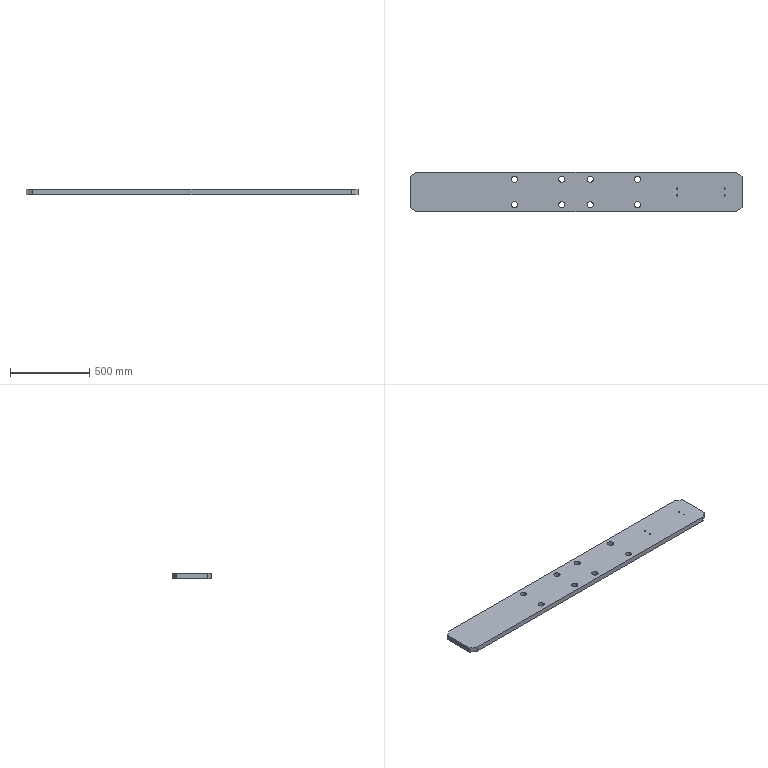Part | SolidWorks | features Extrusion 1, HoleWzd 1, LPattern 1 | 1 solid | 34 faces | box 2100 x 250 x 32 mm | volume 16420254 mm3 | cylinder 24 | plane 10 | commonest cylinder face diameters 39 x16 6.8 x8
STEP:
#1=CARTESIAN_POINT('',(936.6,-22.,-16.));
#2=VERTEX_POINT('',#1);
#3=CARTESIAN_POINT('',(943.4,-22.,-16.));
#4=VERTEX_POINT('',#3);
#5=CARTESIAN_POINT('',(940.,-22.,-16.));
#6=DIRECTION('',(0.,0.,1.));
#7=DIRECTION('',(1.,0.,0.));
#8=AXIS2_PLACEMENT_3D('',#5,#6,#7);
#9=CIRCLE('',#8,3.4);
#10=EDGE_CURVE('',#2,#4,#9,.T.);
#11=ORIENTED_EDGE('',*,*,#10,.F.);
#12=CARTESIAN_POINT('',(936.6,-22.,16.));
#13=VERTEX_POINT('',#12);
#14=CARTESIAN_POINT('',(936.6,-22.,16.));
#15=DIRECTION('',(0.,0.,1.));
#16=VECTOR('',#15,1000.);
#17=LINE('',#14,#16);
#18=EDGE_CURVE('',#2,#13,#17,.T.);
#19=ORIENTED_EDGE('',*,*,#18,.T.);
#20=CARTESIAN_POINT('',(943.4,-22.,16.));
#21=VERTEX_POINT('',#20);
#22=CARTESIAN_POINT('',(940.,-22.,16.));
#23=DIRECTION('',(0.,0.,1.));
#24=DIRECTION('',(1.,0.,0.));
#25=AXIS2_PLACEMENT_3D('',#22,#23,#24);
#26=CIRCLE('',#25,3.4);
#27=EDGE_CURVE('',#13,#21,#26,.T.);
#28=ORIENTED_EDGE('',*,*,#27,.T.);
#29=CARTESIAN_POINT('',(943.4,-22.,16.));
#30=DIRECTION('',(0.,0.,1.));
#31=VECTOR('',#30,1000.);
#32=LINE('',#29,#31);
#33=EDGE_CURVE('',#4,#21,#32,.T.);
#34=ORIENTED_EDGE('',*,*,#33,.F.);
#35=EDGE_LOOP('',(#11,#19,#28,#34));
#36=FACE_OUTER_BOUND('',#35,.T.);
#37=CARTESIAN_POINT('',(940.,-22.,16.));
#38=DIRECTION('',(0.,0.,1.));
#39=DIRECTION('',(1.,0.,0.));
#40=AXIS2_PLACEMENT_3D('',#37,#38,#39);
#41=CYLINDRICAL_SURFACE('',#40,3.4);
#42=ADVANCED_FACE('',(#36),#41,.F.);
#43=CARTESIAN_POINT('',(636.6,-22.,-16.));
#44=VERTEX_POINT('',#43);
#45=CARTESIAN_POINT('',(643.4,-22.,-16.));
#46=VERTEX_POINT('',#45);
#47=CARTESIAN_POINT('',(640.,-22.,-16.));
#48=DIRECTION('',(0.,0.,1.));
#49=DIRECTION('',(1.,0.,0.));
#50=AXIS2_PLACEMENT_3D('',#47,#48,#49);
#51=CIRCLE('',#50,3.4);
#52=EDGE_CURVE('',#44,#46,#51,.T.);
#53=ORIENTED_EDGE('',*,*,#52,.F.);
#54=CARTESIAN_POINT('',(636.6,-22.,16.));
#55=VERTEX_POINT('',#54);
#56=CARTESIAN_POINT('',(636.6,-22.,16.));
#57=DIRECTION('',(0.,0.,1.));
#58=VECTOR('',#57,1000.);
#59=LINE('',#56,#58);
#60=EDGE_CURVE('',#44,#55,#59,.T.);
#61=ORIENTED_EDGE('',*,*,#60,.T.);
#62=CARTESIAN_POINT('',(643.4,-22.,16.));
#63=VERTEX_POINT('',#62);
#64=CARTESIAN_POINT('',(640.,-22.,16.));
#65=DIRECTION('',(0.,0.,1.));
#66=DIRECTION('',(1.,0.,0.));
#67=AXIS2_PLACEMENT_3D('',#64,#65,#66);
#68=CIRCLE('',#67,3.4);
#69=EDGE_CURVE('',#55,#63,#68,.T.);
#70=ORIENTED_EDGE('',*,*,#69,.T.);
#71=CARTESIAN_POINT('',(643.4,-22.,16.));
#72=DIRECTION('',(0.,0.,1.));
#73=VECTOR('',#72,1000.);
#74=LINE('',#71,#73);
#75=EDGE_CURVE('',#46,#63,#74,.T.);
#76=ORIENTED_EDGE('',*,*,#75,.F.);
#77=EDGE_LOOP('',(#53,#61,#70,#76));
#78=FACE_OUTER_BOUND('',#77,.T.);
#79=CARTESIAN_POINT('',(640.,-22.,16.));
#80=DIRECTION('',(0.,0.,1.));
#81=DIRECTION('',(1.,0.,0.));
#82=AXIS2_PLACEMENT_3D('',#79,#80,#81);
#83=CYLINDRICAL_SURFACE('',#82,3.4);
#84=ADVANCED_FACE('',(#78),#83,.F.);
#85=CARTESIAN_POINT('',(936.6,22.,-16.));
#86=VERTEX_POINT('',#85);
#87=CARTESIAN_POINT('',(943.4,22.,-16.));
#88=VERTEX_POINT('',#87);
#89=CARTESIAN_POINT('',(940.,22.,-16.));
#90=DIRECTION('',(0.,0.,1.));
#91=DIRECTION('',(1.,0.,0.));
#92=AXIS2_PLACEMENT_3D('',#89,#90,#91);
#93=CIRCLE('',#92,3.4);
#94=EDGE_CURVE('',#86,#88,#93,.T.);
#95=ORIENTED_EDGE('',*,*,#94,.F.);
#96=CARTESIAN_POINT('',(936.6,22.,16.));
#97=VERTEX_POINT('',#96);
#98=CARTESIAN_POINT('',(936.6,22.,16.));
#99=DIRECTION('',(0.,0.,1.));
#100=VECTOR('',#99,1000.);
#101=LINE('',#98,#100);
#102=EDGE_CURVE('',#86,#97,#101,.T.);
#103=ORIENTED_EDGE('',*,*,#102,.T.);
#104=CARTESIAN_POINT('',(943.4,22.,16.));
#105=VERTEX_POINT('',#104);
#106=CARTESIAN_POINT('',(940.,22.,16.));
#107=DIRECTION('',(0.,0.,1.));
#108=DIRECTION('',(1.,0.,0.));
#109=AXIS2_PLACEMENT_3D('',#106,#107,#108);
#110=CIRCLE('',#109,3.4);
#111=EDGE_CURVE('',#97,#105,#110,.T.);
#112=ORIENTED_EDGE('',*,*,#111,.T.);
#113=CARTESIAN_POINT('',(943.4,22.,16.));
#114=DIRECTION('',(0.,0.,1.));
#115=VECTOR('',#114,1000.);
#116=LINE('',#113,#115);
#117=EDGE_CURVE('',#88,#105,#116,.T.);
#118=ORIENTED_EDGE('',*,*,#117,.F.);
#119=EDGE_LOOP('',(#95,#103,#112,#118));
#120=FACE_OUTER_BOUND('',#119,.T.);
#121=CARTESIAN_POINT('',(940.,22.,16.));
#122=DIRECTION('',(0.,0.,1.));
#123=DIRECTION('',(1.,0.,0.));
#124=AXIS2_PLACEMENT_3D('',#121,#122,#123);
#125=CYLINDRICAL_SURFACE('',#124,3.4);
#126=ADVANCED_FACE('',(#120),#125,.F.);
#127=CARTESIAN_POINT('',(636.6,22.,-16.));
#128=VERTEX_POINT('',#127);
#129=CARTESIAN_POINT('',(643.4,22.,-16.));
#130=VERTEX_POINT('',#129);
#131=CARTESIAN_POINT('',(640.,22.,-16.));
#132=DIRECTION('',(0.,0.,1.));
#133=DIRECTION('',(1.,0.,0.));
#134=AXIS2_PLACEMENT_3D('',#131,#132,#133);
#135=CIRCLE('',#134,3.4);
#136=EDGE_CURVE('',#128,#130,#135,.T.);
#137=ORIENTED_EDGE('',*,*,#136,.F.);
#138=CARTESIAN_POINT('',(636.6,22.,16.));
#139=VERTEX_POINT('',#138);
#140=CARTESIAN_POINT('',(636.6,22.,16.));
#141=DIRECTION('',(0.,0.,1.));
#142=VECTOR('',#141,1000.);
#143=LINE('',#140,#142);
#144=EDGE_CURVE('',#128,#139,#143,.T.);
#145=ORIENTED_EDGE('',*,*,#144,.T.);
#146=CARTESIAN_POINT('',(643.4,22.,16.));
#147=VERTEX_POINT('',#146);
#148=CARTESIAN_POINT('',(640.,22.,16.));
#149=DIRECTION('',(0.,0.,1.));
#150=DIRECTION('',(1.,0.,0.));
#151=AXIS2_PLACEMENT_3D('',#148,#149,#150);
#152=CIRCLE('',#151,3.4);
#153=EDGE_CURVE('',#139,#147,#152,.T.);
#154=ORIENTED_EDGE('',*,*,#153,.T.);
#155=CARTESIAN_POINT('',(643.4,22.,16.));
#156=DIRECTION('',(0.,0.,1.));
#157=VECTOR('',#156,1000.);
#158=LINE('',#155,#157);
#159=EDGE_CURVE('',#130,#147,#158,.T.);
#160=ORIENTED_EDGE('',*,*,#159,.F.);
#161=EDGE_LOOP('',(#137,#145,#154,#160));
#162=FACE_OUTER_BOUND('',#161,.T.);
#163=CARTESIAN_POINT('',(640.,22.,16.));
#164=DIRECTION('',(0.,0.,1.));
#165=DIRECTION('',(1.,0.,0.));
#166=AXIS2_PLACEMENT_3D('',#163,#164,#165);
#167=CYLINDRICAL_SURFACE('',#166,3.4);
#168=ADVANCED_FACE('',(#162),#167,.F.);
#169=CARTESIAN_POINT('',(370.5,80.,16.));
#170=VERTEX_POINT('',#169);
#171=CARTESIAN_POINT('',(409.5,80.,16.));
#172=VERTEX_POINT('',#171);
#173=CARTESIAN_POINT('',(390.,80.,16.));
#174=DIRECTION('',(0.,0.,1.));
#175=DIRECTION('',(-1.,0.,0.));
#176=AXIS2_PLACEMENT_3D('',#173,#174,#175);
#177=CIRCLE('',#176,19.5);
#178=EDGE_CURVE('',#170,#172,#177,.T.);
#179=ORIENTED_EDGE('',*,*,#178,.T.);
#180=CARTESIAN_POINT('',(409.5,80.,-16.));
#181=VERTEX_POINT('',#180);
#182=CARTESIAN_POINT('',(409.5,80.,16.));
#183=DIRECTION('',(0.,0.,-1.));
#184=VECTOR('',#183,1000.);
#185=LINE('',#182,#184);
#186=EDGE_CURVE('',#172,#181,#185,.T.);
#187=ORIENTED_EDGE('',*,*,#186,.T.);
#188=CARTESIAN_POINT('',(370.5,80.,-16.));
#189=VERTEX_POINT('',#188);
#190=CARTESIAN_POINT('',(390.,80.,-16.));
#191=DIRECTION('',(0.,0.,1.));
#192=DIRECTION('',(-1.,0.,0.));
#193=AXIS2_PLACEMENT_3D('',#190,#191,#192);
#194=CIRCLE('',#193,19.5);
#195=EDGE_CURVE('',#189,#181,#194,.T.);
#196=ORIENTED_EDGE('',*,*,#195,.F.);
#197=CARTESIAN_POINT('',(370.5,80.,16.));
#198=DIRECTION('',(0.,0.,-1.));
#199=VECTOR('',#198,1000.);
#200=LINE('',#197,#199);
#201=EDGE_CURVE('',#170,#189,#200,.T.);
#202=ORIENTED_EDGE('',*,*,#201,.F.);
#203=EDGE_LOOP('',(#179,#187,#196,#202));
#204=FACE_OUTER_BOUND('',#203,.T.);
#205=CARTESIAN_POINT('',(390.,80.,16.));
#206=DIRECTION('',(0.,0.,-1.));
#207=DIRECTION('',(-1.,0.,0.));
#208=AXIS2_PLACEMENT_3D('',#205,#206,#207);
#209=CYLINDRICAL_SURFACE('',#208,19.5);
#210=ADVANCED_FACE('',(#204),#209,.F.);
#211=CARTESIAN_POINT('',(70.5,80.,16.));
#212=VERTEX_POINT('',#211);
#213=CARTESIAN_POINT('',(109.5,80.,16.));
#214=VERTEX_POINT('',#213);
#215=CARTESIAN_POINT('',(90.,80.,16.));
#216=DIRECTION('',(0.,0.,1.));
#217=DIRECTION('',(-1.,0.,0.));
#218=AXIS2_PLACEMENT_3D('',#215,#216,#217);
#219=CIRCLE('',#218,19.5);
#220=EDGE_CURVE('',#212,#214,#219,.T.);
#221=ORIENTED_EDGE('',*,*,#220,.T.);
#222=CARTESIAN_POINT('',(109.5,80.,-16.));
#223=VERTEX_POINT('',#222);
#224=CARTESIAN_POINT('',(109.5,80.,16.));
#225=DIRECTION('',(0.,0.,-1.));
#226=VECTOR('',#225,1000.);
#227=LINE('',#224,#226);
#228=EDGE_CURVE('',#214,#223,#227,.T.);
#229=ORIENTED_EDGE('',*,*,#228,.T.);
#230=CARTESIAN_POINT('',(70.5,80.,-16.));
#231=VERTEX_POINT('',#230);
#232=CARTESIAN_POINT('',(90.,80.,-16.));
#233=DIRECTION('',(0.,0.,1.));
#234=DIRECTION('',(-1.,0.,0.));
#235=AXIS2_PLACEMENT_3D('',#232,#233,#234);
#236=CIRCLE('',#235,19.5);
#237=EDGE_CURVE('',#231,#223,#236,.T.);
#238=ORIENTED_EDGE('',*,*,#237,.F.);
#239=CARTESIAN_POINT('',(70.5,80.,16.));
#240=DIRECTION('',(0.,0.,-1.));
#241=VECTOR('',#240,1000.);
#242=LINE('',#239,#241);
#243=EDGE_CURVE('',#212,#231,#242,.T.);
#244=ORIENTED_EDGE('',*,*,#243,.F.);
#245=EDGE_LOOP('',(#221,#229,#238,#244));
#246=FACE_OUTER_BOUND('',#245,.T.);
#247=CARTESIAN_POINT('',(90.,80.,16.));
#248=DIRECTION('',(0.,0.,-1.));
#249=DIRECTION('',(-1.,0.,0.));
#250=AXIS2_PLACEMENT_3D('',#247,#248,#249);
#251=CYLINDRICAL_SURFACE('',#250,19.5);
#252=ADVANCED_FACE('',(#246),#251,.F.);
#253=CARTESIAN_POINT('',(70.5,-80.,16.));
#254=VERTEX_POINT('',#253);
#255=CARTESIAN_POINT('',(109.5,-80.,16.));
#256=VERTEX_POINT('',#255);
#257=CARTESIAN_POINT('',(90.,-80.,16.));
#258=DIRECTION('',(0.,0.,1.));
#259=DIRECTION('',(1.,0.,0.));
#260=AXIS2_PLACEMENT_3D('',#257,#258,#259);
#261=CIRCLE('',#260,19.5);
#262=EDGE_CURVE('',#254,#256,#261,.T.);
#263=ORIENTED_EDGE('',*,*,#262,.T.);
#264=CARTESIAN_POINT('',(109.5,-80.,-16.));
#265=VERTEX_POINT('',#264);
#266=CARTESIAN_POINT('',(109.5,-80.,16.));
#267=DIRECTION('',(0.,0.,-1.));
#268=VECTOR('',#267,1000.);
#269=LINE('',#266,#268);
#270=EDGE_CURVE('',#256,#265,#269,.T.);
#271=ORIENTED_EDGE('',*,*,#270,.T.);
#272=CARTESIAN_POINT('',(70.5,-80.,-16.));
#273=VERTEX_POINT('',#272);
#274=CARTESIAN_POINT('',(90.,-80.,-16.));
#275=DIRECTION('',(0.,0.,1.));
#276=DIRECTION('',(1.,0.,0.));
#277=AXIS2_PLACEMENT_3D('',#274,#275,#276);
#278=CIRCLE('',#277,19.5);
#279=EDGE_CURVE('',#273,#265,#278,.T.);
#280=ORIENTED_EDGE('',*,*,#279,.F.);
#281=CARTESIAN_POINT('',(70.5,-80.,16.));
#282=DIRECTION('',(0.,0.,-1.));
#283=VECTOR('',#282,1000.);
#284=LINE('',#281,#283);
#285=EDGE_CURVE('',#254,#273,#284,.T.);
#286=ORIENTED_EDGE('',*,*,#285,.F.);
#287=EDGE_LOOP('',(#263,#271,#280,#286));
#288=FACE_OUTER_BOUND('',#287,.T.);
#289=CARTESIAN_POINT('',(90.,-80.,16.));
#290=DIRECTION('',(0.,0.,-1.));
#291=DIRECTION('',(-1.,0.,0.));
#292=AXIS2_PLACEMENT_3D('',#289,#290,#291);
#293=CYLINDRICAL_SURFACE('',#292,19.5);
#294=ADVANCED_FACE('',(#288),#293,.F.);
#295=CARTESIAN_POINT('',(370.5,-80.,16.));
#296=VERTEX_POINT('',#295);
#297=CARTESIAN_POINT('',(409.5,-80.,16.));
#298=VERTEX_POINT('',#297);
#299=CARTESIAN_POINT('',(390.,-80.,16.));
#300=DIRECTION('',(0.,0.,1.));
#301=DIRECTION('',(1.,0.,0.));
#302=AXIS2_PLACEMENT_3D('',#299,#300,#301);
#303=CIRCLE('',#302,19.5);
#304=EDGE_CURVE('',#296,#298,#303,.T.);
#305=ORIENTED_EDGE('',*,*,#304,.T.);
#306=CARTESIAN_POINT('',(409.5,-80.,-16.));
#307=VERTEX_POINT('',#306);
#308=CARTESIAN_POINT('',(409.5,-80.,16.));
#309=DIRECTION('',(0.,0.,-1.));
#310=VECTOR('',#309,1000.);
#311=LINE('',#308,#310);
#312=EDGE_CURVE('',#298,#307,#311,.T.);
#313=ORIENTED_EDGE('',*,*,#312,.T.);
#314=CARTESIAN_POINT('',(370.5,-80.,-16.));
#315=VERTEX_POINT('',#314);
#316=CARTESIAN_POINT('',(390.,-80.,-16.));
#317=DIRECTION('',(0.,0.,1.));
#318=DIRECTION('',(1.,0.,0.));
#319=AXIS2_PLACEMENT_3D('',#316,#317,#318);
#320=CIRCLE('',#319,19.5);
#321=EDGE_CURVE('',#315,#307,#320,.T.);
#322=ORIENTED_EDGE('',*,*,#321,.F.);
#323=CARTESIAN_POINT('',(370.5,-80.,16.));
#324=DIRECTION('',(0.,0.,-1.));
#325=VECTOR('',#324,1000.);
#326=LINE('',#323,#325);
#327=EDGE_CURVE('',#296,#315,#326,.T.);
#328=ORIENTED_EDGE('',*,*,#327,.F.);
#329=EDGE_LOOP('',(#305,#313,#322,#328));
#330=FACE_OUTER_BOUND('',#329,.T.);
#331=CARTESIAN_POINT('',(390.,-80.,16.));
#332=DIRECTION('',(0.,0.,-1.));
#333=DIRECTION('',(-1.,0.,0.));
#334=AXIS2_PLACEMENT_3D('',#331,#332,#333);
#335=CYLINDRICAL_SURFACE('',#334,19.5);
#336=ADVANCED_FACE('',(#330),#335,.F.);
#337=CARTESIAN_POINT('',(-409.5,-80.,16.));
#338=VERTEX_POINT('',#337);
#339=CARTESIAN_POINT('',(-370.5,-80.,16.));
#340=VERTEX_POINT('',#339);
#341=CARTESIAN_POINT('',(-390.,-80.,16.));
#342=DIRECTION('',(0.,0.,1.));
#343=DIRECTION('',(-1.,0.,0.));
#344=AXIS2_PLACEMENT_3D('',#341,#342,#343);
#345=CIRCLE('',#344,19.5);
#346=EDGE_CURVE('',#338,#340,#345,.T.);
#347=ORIENTED_EDGE('',*,*,#346,.T.);
#348=CARTESIAN_POINT('',(-370.5,-80.,-16.));
#349=VERTEX_POINT('',#348);
#350=CARTESIAN_POINT('',(-370.5,-80.,16.));
#351=DIRECTION('',(0.,0.,-1.));
#352=VECTOR('',#351,1000.);
#353=LINE('',#350,#352);
#354=EDGE_CURVE('',#340,#349,#353,.T.);
#355=ORIENTED_EDGE('',*,*,#354,.T.);
#356=CARTESIAN_POINT('',(-409.5,-80.,-16.));
#357=VERTEX_POINT('',#356);
#358=CARTESIAN_POINT('',(-390.,-80.,-16.));
#359=DIRECTION('',(0.,0.,1.));
#360=DIRECTION('',(-1.,0.,0.));
#361=AXIS2_PLACEMENT_3D('',#358,#359,#360);
#362=CIRCLE('',#361,19.5);
#363=EDGE_CURVE('',#357,#349,#362,.T.);
#364=ORIENTED_EDGE('',*,*,#363,.F.);
#365=CARTESIAN_POINT('',(-409.5,-80.,16.));
#366=DIRECTION('',(0.,0.,-1.));
#367=VECTOR('',#366,1000.);
#368=LINE('',#365,#367);
#369=EDGE_CURVE('',#338,#357,#368,.T.);
#370=ORIENTED_EDGE('',*,*,#369,.F.);
#371=EDGE_LOOP('',(#347,#355,#364,#370));
#372=FACE_OUTER_BOUND('',#371,.T.);
#373=CARTESIAN_POINT('',(-390.,-80.,16.));
#374=DIRECTION('',(0.,0.,-1.));
#375=DIRECTION('',(-1.,0.,0.));
#376=AXIS2_PLACEMENT_3D('',#373,#374,#375);
#377=CYLINDRICAL_SURFACE('',#376,19.5);
#378=ADVANCED_FACE('',(#372),#377,.F.);
#379=CARTESIAN_POINT('',(-109.5,-80.,16.));
#380=VERTEX_POINT('',#379);
#381=CARTESIAN_POINT('',(-70.5,-80.,16.));
#382=VERTEX_POINT('',#381);
#383=CARTESIAN_POINT('',(-90.,-80.,16.));
#384=DIRECTION('',(0.,0.,1.));
#385=DIRECTION('',(-1.,0.,0.));
#386=AXIS2_PLACEMENT_3D('',#383,#384,#385);
#387=CIRCLE('',#386,19.5);
#388=EDGE_CURVE('',#380,#382,#387,.T.);
#389=ORIENTED_EDGE('',*,*,#388,.T.);
#390=CARTESIAN_POINT('',(-70.5,-80.,-16.));
#391=VERTEX_POINT('',#390);
#392=CARTESIAN_POINT('',(-70.5,-80.,16.));
#393=DIRECTION('',(0.,0.,-1.));
#394=VECTOR('',#393,1000.);
#395=LINE('',#392,#394);
#396=EDGE_CURVE('',#382,#391,#395,.T.);
#397=ORIENTED_EDGE('',*,*,#396,.T.);
#398=CARTESIAN_POINT('',(-109.5,-80.,-16.));
#399=VERTEX_POINT('',#398);
#400=CARTESIAN_POINT('',(-90.,-80.,-16.));
#401=DIRECTION('',(0.,0.,1.));
#402=DIRECTION('',(-1.,0.,0.));
#403=AXIS2_PLACEMENT_3D('',#400,#401,#402);
#404=CIRCLE('',#403,19.5);
#405=EDGE_CURVE('',#399,#391,#404,.T.);
#406=ORIENTED_EDGE('',*,*,#405,.F.);
#407=CARTESIAN_POINT('',(-109.5,-80.,16.));
#408=DIRECTION('',(0.,0.,-1.));
#409=VECTOR('',#408,1000.);
#410=LINE('',#407,#409);
#411=EDGE_CURVE('',#380,#399,#410,.T.);
#412=ORIENTED_EDGE('',*,*,#411,.F.);
#413=EDGE_LOOP('',(#389,#397,#406,#412));
#414=FACE_OUTER_BOUND('',#413,.T.);
#415=CARTESIAN_POINT('',(-90.,-80.,16.));
#416=DIRECTION('',(0.,0.,-1.));
#417=DIRECTION('',(-1.,0.,0.));
#418=AXIS2_PLACEMENT_3D('',#415,#416,#417);
#419=CYLINDRICAL_SURFACE('',#418,19.5);
#420=ADVANCED_FACE('',(#414),#419,.F.);
#421=CARTESIAN_POINT('',(-109.5,80.,16.));
#422=VERTEX_POINT('',#421);
#423=CARTESIAN_POINT('',(-70.5,80.,16.));
#424=VERTEX_POINT('',#423);
#425=CARTESIAN_POINT('',(-90.,80.,16.));
#426=DIRECTION('',(0.,0.,1.));
#427=DIRECTION('',(1.,0.,0.));
#428=AXIS2_PLACEMENT_3D('',#425,#426,#427);
#429=CIRCLE('',#428,19.5);
#430=EDGE_CURVE('',#422,#424,#429,.T.);
#431=ORIENTED_EDGE('',*,*,#430,.T.);
#432=CARTESIAN_POINT('',(-70.5,80.,-16.));
#433=VERTEX_POINT('',#432);
#434=CARTESIAN_POINT('',(-70.5,80.,16.));
#435=DIRECTION('',(0.,0.,-1.));
#436=VECTOR('',#435,1000.);
#437=LINE('',#434,#436);
#438=EDGE_CURVE('',#424,#433,#437,.T.);
#439=ORIENTED_EDGE('',*,*,#438,.T.);
#440=CARTESIAN_POINT('',(-109.5,80.,-16.));
#441=VERTEX_POINT('',#440);
#442=CARTESIAN_POINT('',(-90.,80.,-16.));
#443=DIRECTION('',(0.,0.,1.));
#444=DIRECTION('',(1.,0.,0.));
#445=AXIS2_PLACEMENT_3D('',#442,#443,#444);
#446=CIRCLE('',#445,19.5);
#447=EDGE_CURVE('',#441,#433,#446,.T.);
#448=ORIENTED_EDGE('',*,*,#447,.F.);
#449=CARTESIAN_POINT('',(-109.5,80.,16.));
#450=DIRECTION('',(0.,0.,-1.));
#451=VECTOR('',#450,1000.);
#452=LINE('',#449,#451);
#453=EDGE_CURVE('',#422,#441,#452,.T.);
#454=ORIENTED_EDGE('',*,*,#453,.F.);
#455=EDGE_LOOP('',(#431,#439,#448,#454));
#456=FACE_OUTER_BOUND('',#455,.T.);
#457=CARTESIAN_POINT('',(-90.,80.,16.));
#458=DIRECTION('',(0.,0.,-1.));
#459=DIRECTION('',(-1.,0.,0.));
#460=AXIS2_PLACEMENT_3D('',#457,#458,#459);
#461=CYLINDRICAL_SURFACE('',#460,19.5);
#462=ADVANCED_FACE('',(#456),#461,.F.);
#463=CARTESIAN_POINT('',(-409.5,80.,16.));
#464=VERTEX_POINT('',#463);
#465=CARTESIAN_POINT('',(-370.5,80.,16.));
#466=VERTEX_POINT('',#465);
#467=CARTESIAN_POINT('',(-390.,80.,16.));
#468=DIRECTION('',(0.,0.,1.));
#469=DIRECTION('',(1.,0.,0.));
#470=AXIS2_PLACEMENT_3D('',#467,#468,#469);
#471=CIRCLE('',#470,19.5);
#472=EDGE_CURVE('',#464,#466,#471,.T.);
#473=ORIENTED_EDGE('',*,*,#472,.T.);
#474=CARTESIAN_POINT('',(-370.5,80.,-16.));
#475=VERTEX_POINT('',#474);
#476=CARTESIAN_POINT('',(-370.5,80.,16.));
#477=DIRECTION('',(0.,0.,-1.));
#478=VECTOR('',#477,1000.);
#479=LINE('',#476,#478);
#480=EDGE_CURVE('',#466,#475,#479,.T.);
#481=ORIENTED_EDGE('',*,*,#480,.T.);
#482=CARTESIAN_POINT('',(-409.5,80.,-16.));
#483=VERTEX_POINT('',#482);
#484=CARTESIAN_POINT('',(-390.,80.,-16.));
#485=DIRECTION('',(0.,0.,1.));
#486=DIRECTION('',(1.,0.,0.));
#487=AXIS2_PLACEMENT_3D('',#484,#485,#486);
#488=CIRCLE('',#487,19.5);
#489=EDGE_CURVE('',#483,#475,#488,.T.);
#490=ORIENTED_EDGE('',*,*,#489,.F.);
#491=CARTESIAN_POINT('',(-409.5,80.,16.));
#492=DIRECTION('',(0.,0.,-1.));
#493=VECTOR('',#492,1000.);
#494=LINE('',#491,#493);
#495=EDGE_CURVE('',#464,#483,#494,.T.);
#496=ORIENTED_EDGE('',*,*,#495,.F.);
#497=EDGE_LOOP('',(#473,#481,#490,#496));
#498=FACE_OUTER_BOUND('',#497,.T.);
#499=CARTESIAN_POINT('',(-390.,80.,16.));
#500=DIRECTION('',(0.,0.,-1.));
#501=DIRECTION('',(-1.,0.,0.));
#502=AXIS2_PLACEMENT_3D('',#499,#500,#501);
#503=CYLINDRICAL_SURFACE('',#502,19.5);
#504=ADVANCED_FACE('',(#498),#503,.F.);
#505=CARTESIAN_POINT('',(940.,22.,16.));
#506=DIRECTION('',(0.,0.,1.));
#507=DIRECTION('',(1.,0.,0.));
#508=AXIS2_PLACEMENT_3D('',#505,#506,#507);
#509=CIRCLE('',#508,3.4);
#510=EDGE_CURVE('',#105,#97,#509,.T.);
#511=ORIENTED_EDGE('',*,*,#510,.F.);
#512=ORIENTED_EDGE('',*,*,#111,.F.);
#513=EDGE_LOOP('',(#511,#512));
#514=FACE_BOUND('',#513,.T.);
#515=CARTESIAN_POINT('',(640.,22.,16.));
#516=DIRECTION('',(0.,0.,1.));
#517=DIRECTION('',(1.,0.,0.));
#518=AXIS2_PLACEMENT_3D('',#515,#516,#517);
#519=CIRCLE('',#518,3.4);
#520=EDGE_CURVE('',#147,#139,#519,.T.);
#521=ORIENTED_EDGE('',*,*,#520,.F.);
#522=ORIENTED_EDGE('',*,*,#153,.F.);
#523=EDGE_LOOP('',(#521,#522));
#524=FACE_BOUND('',#523,.T.);
#525=ORIENTED_EDGE('',*,*,#220,.F.);
#526=CARTESIAN_POINT('',(90.,80.,16.));
#527=DIRECTION('',(0.,0.,1.));
#528=DIRECTION('',(-1.,0.,0.));
#529=AXIS2_PLACEMENT_3D('',#526,#527,#528);
#530=CIRCLE('',#529,19.5);
#531=EDGE_CURVE('',#214,#212,#530,.T.);
#532=ORIENTED_EDGE('',*,*,#531,.F.);
#533=EDGE_LOOP('',(#525,#532));
#534=FACE_BOUND('',#533,.T.);
#535=ORIENTED_EDGE('',*,*,#304,.F.);
#536=CARTESIAN_POINT('',(390.,-80.,16.));
#537=DIRECTION('',(0.,0.,1.));
#538=DIRECTION('',(1.,0.,0.));
#539=AXIS2_PLACEMENT_3D('',#536,#537,#538);
#540=CIRCLE('',#539,19.5);
#541=EDGE_CURVE('',#298,#296,#540,.T.);
#542=ORIENTED_EDGE('',*,*,#541,.F.);
#543=EDGE_LOOP('',(#535,#542));
#544=FACE_BOUND('',#543,.T.);
#545=ORIENTED_EDGE('',*,*,#388,.F.);
#546=CARTESIAN_POINT('',(-90.,-80.,16.));
#547=DIRECTION('',(0.,0.,1.));
#548=DIRECTION('',(-1.,0.,0.));
#549=AXIS2_PLACEMENT_3D('',#546,#547,#548);
#550=CIRCLE('',#549,19.5);
#551=EDGE_CURVE('',#382,#380,#550,.T.);
#552=ORIENTED_EDGE('',*,*,#551,.F.);
#553=EDGE_LOOP('',(#545,#552));
#554=FACE_BOUND('',#553,.T.);
#555=ORIENTED_EDGE('',*,*,#472,.F.);
#556=CARTESIAN_POINT('',(-390.,80.,16.));
#557=DIRECTION('',(0.,0.,1.));
#558=DIRECTION('',(1.,0.,0.));
#559=AXIS2_PLACEMENT_3D('',#556,#557,#558);
#560=CIRCLE('',#559,19.5);
#561=EDGE_CURVE('',#466,#464,#560,.T.);
#562=ORIENTED_EDGE('',*,*,#561,.F.);
#563=EDGE_LOOP('',(#555,#562));
#564=FACE_BOUND('',#563,.T.);
#565=CARTESIAN_POINT('',(1006.699,-125.,16.));
#566=VERTEX_POINT('',#565);
#567=CARTESIAN_POINT('',(1050.,-100.,16.));
#568=VERTEX_POINT('',#567);
#569=CARTESIAN_POINT('',(1050.,-100.,16.));
#570=DIRECTION('',(0.866,0.5,0.));
#571=VECTOR('',#570,1000.);
#572=LINE('',#569,#571);
#573=EDGE_CURVE('',#566,#568,#572,.T.);
#574=ORIENTED_EDGE('',*,*,#573,.T.);
#575=CARTESIAN_POINT('',(1050.,100.,16.));
#576=VERTEX_POINT('',#575);
#577=CARTESIAN_POINT('',(1050.,100.,16.));
#578=DIRECTION('',(0.,1.,0.));
#579=VECTOR('',#578,1000.);
#580=LINE('',#577,#579);
#581=EDGE_CURVE('',#568,#576,#580,.T.);
#582=ORIENTED_EDGE('',*,*,#581,.T.);
#583=CARTESIAN_POINT('',(1006.699,125.,16.));
#584=VERTEX_POINT('',#583);
#585=CARTESIAN_POINT('',(1050.,100.,16.));
#586=DIRECTION('',(-0.866,0.5,0.));
#587=VECTOR('',#586,1000.);
#588=LINE('',#585,#587);
#589=EDGE_CURVE('',#576,#584,#588,.T.);
#590=ORIENTED_EDGE('',*,*,#589,.T.);
#591=CARTESIAN_POINT('',(-1006.699,125.,16.));
#592=VERTEX_POINT('',#591);
#593=CARTESIAN_POINT('',(-1006.699,125.,16.));
#594=DIRECTION('',(-1.,0.,0.));
#595=VECTOR('',#594,1000.);
#596=LINE('',#593,#595);
#597=EDGE_CURVE('',#584,#592,#596,.T.);
#598=ORIENTED_EDGE('',*,*,#597,.T.);
#599=CARTESIAN_POINT('',(-1050.,100.,16.));
#600=VERTEX_POINT('',#599);
#601=CARTESIAN_POINT('',(-1050.,100.,16.));
#602=DIRECTION('',(-0.866,-0.5,0.));
#603=VECTOR('',#602,1000.);
#604=LINE('',#601,#603);
#605=EDGE_CURVE('',#592,#600,#604,.T.);
#606=ORIENTED_EDGE('',*,*,#605,.T.);
#607=CARTESIAN_POINT('',(-1050.,-100.,16.));
#608=VERTEX_POINT('',#607);
#609=CARTESIAN_POINT('',(-1050.,100.,16.));
#610=DIRECTION('',(0.,-1.,0.));
#611=VECTOR('',#610,1000.);
#612=LINE('',#609,#611);
#613=EDGE_CURVE('',#600,#608,#612,.T.);
#614=ORIENTED_EDGE('',*,*,#613,.T.);
#615=CARTESIAN_POINT('',(-1006.699,-125.,16.));
#616=VERTEX_POINT('',#615);
#617=CARTESIAN_POINT('',(-1050.,-100.,16.));
#618=DIRECTION('',(0.866,-0.5,0.));
#619=VECTOR('',#618,1000.);
#620=LINE('',#617,#619);
#621=EDGE_CURVE('',#608,#616,#620,.T.);
#622=ORIENTED_EDGE('',*,*,#621,.T.);
#623=CARTESIAN_POINT('',(-1006.699,-125.,16.));
#624=DIRECTION('',(1.,0.,0.));
#625=VECTOR('',#624,1000.);
#626=LINE('',#623,#625);
#627=EDGE_CURVE('',#616,#566,#626,.T.);
#628=ORIENTED_EDGE('',*,*,#627,.T.);
#629=EDGE_LOOP('',(#574,#582,#590,#598,#606,#614,#622,#628));
#630=FACE_OUTER_BOUND('',#629,.T.);
#631=ORIENTED_EDGE('',*,*,#430,.F.);
#632=CARTESIAN_POINT('',(-90.,80.,16.));
#633=DIRECTION('',(0.,0.,1.));
#634=DIRECTION('',(1.,0.,0.));
#635=AXIS2_PLACEMENT_3D('',#632,#633,#634);
#636=CIRCLE('',#635,19.5);
#637=EDGE_CURVE('',#424,#422,#636,.T.);
#638=ORIENTED_EDGE('',*,*,#637,.F.);
#639=EDGE_LOOP('',(#631,#638));
#640=FACE_BOUND('',#639,.T.);
#641=ORIENTED_EDGE('',*,*,#346,.F.);
#642=CARTESIAN_POINT('',(-390.,-80.,16.));
#643=DIRECTION('',(0.,0.,1.));
#644=DIRECTION('',(-1.,0.,0.));
#645=AXIS2_PLACEMENT_3D('',#642,#643,#644);
#646=CIRCLE('',#645,19.5);
#647=EDGE_CURVE('',#340,#338,#646,.T.);
#648=ORIENTED_EDGE('',*,*,#647,.F.);
#649=EDGE_LOOP('',(#641,#648));
#650=FACE_BOUND('',#649,.T.);
#651=ORIENTED_EDGE('',*,*,#262,.F.);
#652=CARTESIAN_POINT('',(90.,-80.,16.));
#653=DIRECTION('',(0.,0.,1.));
#654=DIRECTION('',(1.,0.,0.));
#655=AXIS2_PLACEMENT_3D('',#652,#653,#654);
#656=CIRCLE('',#655,19.5);
#657=EDGE_CURVE('',#256,#254,#656,.T.);
#658=ORIENTED_EDGE('',*,*,#657,.F.);
#659=EDGE_LOOP('',(#651,#658));
#660=FACE_BOUND('',#659,.T.);
#661=ORIENTED_EDGE('',*,*,#178,.F.);
#662=CARTESIAN_POINT('',(390.,80.,16.));
#663=DIRECTION('',(0.,0.,1.));
#664=DIRECTION('',(-1.,0.,0.));
#665=AXIS2_PLACEMENT_3D('',#662,#663,#664);
#666=CIRCLE('',#665,19.5);
#667=EDGE_CURVE('',#172,#170,#666,.T.);
#668=ORIENTED_EDGE('',*,*,#667,.F.);
#669=EDGE_LOOP('',(#661,#668));
#670=FACE_BOUND('',#669,.T.);
#671=CARTESIAN_POINT('',(640.,-22.,16.));
#672=DIRECTION('',(0.,0.,1.));
#673=DIRECTION('',(1.,0.,0.));
#674=AXIS2_PLACEMENT_3D('',#671,#672,#673);
#675=CIRCLE('',#674,3.4);
#676=EDGE_CURVE('',#63,#55,#675,.T.);
#677=ORIENTED_EDGE('',*,*,#676,.F.);
#678=ORIENTED_EDGE('',*,*,#69,.F.);
#679=EDGE_LOOP('',(#677,#678));
#680=FACE_BOUND('',#679,.T.);
#681=CARTESIAN_POINT('',(940.,-22.,16.));
#682=DIRECTION('',(0.,0.,1.));
#683=DIRECTION('',(1.,0.,0.));
#684=AXIS2_PLACEMENT_3D('',#681,#682,#683);
#685=CIRCLE('',#684,3.4);
#686=EDGE_CURVE('',#21,#13,#685,.T.);
#687=ORIENTED_EDGE('',*,*,#686,.F.);
#688=ORIENTED_EDGE('',*,*,#27,.F.);
#689=EDGE_LOOP('',(#687,#688));
#690=FACE_BOUND('',#689,.T.);
#691=CARTESIAN_POINT('',(0.,-706.218,16.));
#692=DIRECTION('',(0.,0.,1.));
#693=DIRECTION('',(1.,0.,0.));
#694=AXIS2_PLACEMENT_3D('',#691,#692,#693);
#695=PLANE('',#694);
#696=ADVANCED_FACE('',(#514,#524,#534,#544,#554,#564,#630,#640,#650,#660,#670,#680,#690),#695,.T.);
#697=CARTESIAN_POINT('',(940.,22.,-16.));
#698=DIRECTION('',(0.,0.,1.));
#699=DIRECTION('',(1.,0.,0.));
#700=AXIS2_PLACEMENT_3D('',#697,#698,#699);
#701=CIRCLE('',#700,3.4);
#702=EDGE_CURVE('',#88,#86,#701,.T.);
#703=ORIENTED_EDGE('',*,*,#702,.T.);
#704=ORIENTED_EDGE('',*,*,#94,.T.);
#705=EDGE_LOOP('',(#703,#704));
#706=FACE_BOUND('',#705,.T.);
#707=CARTESIAN_POINT('',(640.,22.,-16.));
#708=DIRECTION('',(0.,0.,1.));
#709=DIRECTION('',(1.,0.,0.));
#710=AXIS2_PLACEMENT_3D('',#707,#708,#709);
#711=CIRCLE('',#710,3.4);
#712=EDGE_CURVE('',#130,#128,#711,.T.);
#713=ORIENTED_EDGE('',*,*,#712,.T.);
#714=ORIENTED_EDGE('',*,*,#136,.T.);
#715=EDGE_LOOP('',(#713,#714));
#716=FACE_BOUND('',#715,.T.);
#717=ORIENTED_EDGE('',*,*,#237,.T.);
#718=CARTESIAN_POINT('',(90.,80.,-16.));
#719=DIRECTION('',(0.,0.,1.));
#720=DIRECTION('',(-1.,0.,0.));
#721=AXIS2_PLACEMENT_3D('',#718,#719,#720);
#722=CIRCLE('',#721,19.5);
#723=EDGE_CURVE('',#223,#231,#722,.T.);
#724=ORIENTED_EDGE('',*,*,#723,.T.);
#725=EDGE_LOOP('',(#717,#724));
#726=FACE_BOUND('',#725,.T.);
#727=ORIENTED_EDGE('',*,*,#321,.T.);
#728=CARTESIAN_POINT('',(390.,-80.,-16.));
#729=DIRECTION('',(0.,0.,1.));
#730=DIRECTION('',(1.,0.,0.));
#731=AXIS2_PLACEMENT_3D('',#728,#729,#730);
#732=CIRCLE('',#731,19.5);
#733=EDGE_CURVE('',#307,#315,#732,.T.);
#734=ORIENTED_EDGE('',*,*,#733,.T.);
#735=EDGE_LOOP('',(#727,#734));
#736=FACE_BOUND('',#735,.T.);
#737=ORIENTED_EDGE('',*,*,#405,.T.);
#738=CARTESIAN_POINT('',(-90.,-80.,-16.));
#739=DIRECTION('',(0.,0.,1.));
#740=DIRECTION('',(-1.,0.,0.));
#741=AXIS2_PLACEMENT_3D('',#738,#739,#740);
#742=CIRCLE('',#741,19.5);
#743=EDGE_CURVE('',#391,#399,#742,.T.);
#744=ORIENTED_EDGE('',*,*,#743,.T.);
#745=EDGE_LOOP('',(#737,#744));
#746=FACE_BOUND('',#745,.T.);
#747=ORIENTED_EDGE('',*,*,#489,.T.);
#748=CARTESIAN_POINT('',(-390.,80.,-16.));
#749=DIRECTION('',(0.,0.,1.));
#750=DIRECTION('',(1.,0.,0.));
#751=AXIS2_PLACEMENT_3D('',#748,#749,#750);
#752=CIRCLE('',#751,19.5);
#753=EDGE_CURVE('',#475,#483,#752,.T.);
#754=ORIENTED_EDGE('',*,*,#753,.T.);
#755=EDGE_LOOP('',(#747,#754));
#756=FACE_BOUND('',#755,.T.);
#757=CARTESIAN_POINT('',(1006.699,-125.,-16.));
#758=VERTEX_POINT('',#757);
#759=CARTESIAN_POINT('',(1050.,-100.,-16.));
#760=VERTEX_POINT('',#759);
#761=CARTESIAN_POINT('',(1050.,-100.,-16.));
#762=DIRECTION('',(0.866,0.5,0.));
#763=VECTOR('',#762,1000.);
#764=LINE('',#761,#763);
#765=EDGE_CURVE('',#758,#760,#764,.T.);
#766=ORIENTED_EDGE('',*,*,#765,.F.);
#767=CARTESIAN_POINT('',(-1006.699,-125.,-16.));
#768=VERTEX_POINT('',#767);
#769=CARTESIAN_POINT('',(-1006.699,-125.,-16.));
#770=DIRECTION('',(1.,0.,0.));
#771=VECTOR('',#770,1000.);
#772=LINE('',#769,#771);
#773=EDGE_CURVE('',#768,#758,#772,.T.);
#774=ORIENTED_EDGE('',*,*,#773,.F.);
#775=CARTESIAN_POINT('',(-1050.,-100.,-16.));
#776=VERTEX_POINT('',#775);
#777=CARTESIAN_POINT('',(-1050.,-100.,-16.));
#778=DIRECTION('',(0.866,-0.5,0.));
#779=VECTOR('',#778,1000.);
#780=LINE('',#777,#779);
#781=EDGE_CURVE('',#776,#768,#780,.T.);
#782=ORIENTED_EDGE('',*,*,#781,.F.);
#783=CARTESIAN_POINT('',(-1050.,100.,-16.));
#784=VERTEX_POINT('',#783);
#785=CARTESIAN_POINT('',(-1050.,100.,-16.));
#786=DIRECTION('',(0.,-1.,0.));
#787=VECTOR('',#786,1000.);
#788=LINE('',#785,#787);
#789=EDGE_CURVE('',#784,#776,#788,.T.);
#790=ORIENTED_EDGE('',*,*,#789,.F.);
#791=CARTESIAN_POINT('',(-1006.699,125.,-16.));
#792=VERTEX_POINT('',#791);
#793=CARTESIAN_POINT('',(-1050.,100.,-16.));
#794=DIRECTION('',(-0.866,-0.5,0.));
#795=VECTOR('',#794,1000.);
#796=LINE('',#793,#795);
#797=EDGE_CURVE('',#792,#784,#796,.T.);
#798=ORIENTED_EDGE('',*,*,#797,.F.);
#799=CARTESIAN_POINT('',(1006.699,125.,-16.));
#800=VERTEX_POINT('',#799);
#801=CARTESIAN_POINT('',(-1006.699,125.,-16.));
#802=DIRECTION('',(-1.,0.,0.));
#803=VECTOR('',#802,1000.);
#804=LINE('',#801,#803);
#805=EDGE_CURVE('',#800,#792,#804,.T.);
#806=ORIENTED_EDGE('',*,*,#805,.F.);
#807=CARTESIAN_POINT('',(1050.,100.,-16.));
#808=VERTEX_POINT('',#807);
#809=CARTESIAN_POINT('',(1050.,100.,-16.));
#810=DIRECTION('',(-0.866,0.5,0.));
#811=VECTOR('',#810,1000.);
#812=LINE('',#809,#811);
#813=EDGE_CURVE('',#808,#800,#812,.T.);
#814=ORIENTED_EDGE('',*,*,#813,.F.);
#815=CARTESIAN_POINT('',(1050.,100.,-16.));
#816=DIRECTION('',(0.,1.,0.));
#817=VECTOR('',#816,1000.);
#818=LINE('',#815,#817);
#819=EDGE_CURVE('',#760,#808,#818,.T.);
#820=ORIENTED_EDGE('',*,*,#819,.F.);
#821=EDGE_LOOP('',(#766,#774,#782,#790,#798,#806,#814,#820));
#822=FACE_OUTER_BOUND('',#821,.T.);
#823=ORIENTED_EDGE('',*,*,#447,.T.);
#824=CARTESIAN_POINT('',(-90.,80.,-16.));
#825=DIRECTION('',(0.,0.,1.));
#826=DIRECTION('',(1.,0.,0.));
#827=AXIS2_PLACEMENT_3D('',#824,#825,#826);
#828=CIRCLE('',#827,19.5);
#829=EDGE_CURVE('',#433,#441,#828,.T.);
#830=ORIENTED_EDGE('',*,*,#829,.T.);
#831=EDGE_LOOP('',(#823,#830));
#832=FACE_BOUND('',#831,.T.);
#833=ORIENTED_EDGE('',*,*,#363,.T.);
#834=CARTESIAN_POINT('',(-390.,-80.,-16.));
#835=DIRECTION('',(0.,0.,1.));
#836=DIRECTION('',(-1.,0.,0.));
#837=AXIS2_PLACEMENT_3D('',#834,#835,#836);
#838=CIRCLE('',#837,19.5);
#839=EDGE_CURVE('',#349,#357,#838,.T.);
#840=ORIENTED_EDGE('',*,*,#839,.T.);
#841=EDGE_LOOP('',(#833,#840));
#842=FACE_BOUND('',#841,.T.);
#843=ORIENTED_EDGE('',*,*,#279,.T.);
#844=CARTESIAN_POINT('',(90.,-80.,-16.));
#845=DIRECTION('',(0.,0.,1.));
#846=DIRECTION('',(1.,0.,0.));
#847=AXIS2_PLACEMENT_3D('',#844,#845,#846);
#848=CIRCLE('',#847,19.5);
#849=EDGE_CURVE('',#265,#273,#848,.T.);
#850=ORIENTED_EDGE('',*,*,#849,.T.);
#851=EDGE_LOOP('',(#843,#850));
#852=FACE_BOUND('',#851,.T.);
#853=ORIENTED_EDGE('',*,*,#195,.T.);
#854=CARTESIAN_POINT('',(390.,80.,-16.));
#855=DIRECTION('',(0.,0.,1.));
#856=DIRECTION('',(-1.,0.,0.));
#857=AXIS2_PLACEMENT_3D('',#854,#855,#856);
#858=CIRCLE('',#857,19.5);
#859=EDGE_CURVE('',#181,#189,#858,.T.);
#860=ORIENTED_EDGE('',*,*,#859,.T.);
#861=EDGE_LOOP('',(#853,#860));
#862=FACE_BOUND('',#861,.T.);
#863=CARTESIAN_POINT('',(640.,-22.,-16.));
#864=DIRECTION('',(0.,0.,1.));
#865=DIRECTION('',(1.,0.,0.));
#866=AXIS2_PLACEMENT_3D('',#863,#864,#865);
#867=CIRCLE('',#866,3.4);
#868=EDGE_CURVE('',#46,#44,#867,.T.);
#869=ORIENTED_EDGE('',*,*,#868,.T.);
#870=ORIENTED_EDGE('',*,*,#52,.T.);
#871=EDGE_LOOP('',(#869,#870));
#872=FACE_BOUND('',#871,.T.);
#873=CARTESIAN_POINT('',(940.,-22.,-16.));
#874=DIRECTION('',(0.,0.,1.));
#875=DIRECTION('',(1.,0.,0.));
#876=AXIS2_PLACEMENT_3D('',#873,#874,#875);
#877=CIRCLE('',#876,3.4);
#878=EDGE_CURVE('',#4,#2,#877,.T.);
#879=ORIENTED_EDGE('',*,*,#878,.T.);
#880=ORIENTED_EDGE('',*,*,#10,.T.);
#881=EDGE_LOOP('',(#879,#880));
#882=FACE_BOUND('',#881,.T.);
#883=CARTESIAN_POINT('',(0.,-706.218,-16.));
#884=DIRECTION('',(0.,0.,1.));
#885=DIRECTION('',(1.,0.,0.));
#886=AXIS2_PLACEMENT_3D('',#883,#884,#885);
#887=PLANE('',#886);
#888=ADVANCED_FACE('',(#706,#716,#726,#736,#746,#756,#822,#832,#842,#852,#862,#872,#882),#887,.F.);
#889=ORIENTED_EDGE('',*,*,#765,.T.);
#890=CARTESIAN_POINT('',(1050.,-100.,16.));
#891=DIRECTION('',(0.,0.,-1.));
#892=VECTOR('',#891,1000.);
#893=LINE('',#890,#892);
#894=EDGE_CURVE('',#568,#760,#893,.T.);
#895=ORIENTED_EDGE('',*,*,#894,.F.);
#896=ORIENTED_EDGE('',*,*,#573,.F.);
#897=CARTESIAN_POINT('',(1006.699,-125.,16.));
#898=DIRECTION('',(0.,0.,-1.));
#899=VECTOR('',#898,1000.);
#900=LINE('',#897,#899);
#901=EDGE_CURVE('',#566,#758,#900,.T.);
#902=ORIENTED_EDGE('',*,*,#901,.T.);
#903=EDGE_LOOP('',(#889,#895,#896,#902));
#904=FACE_OUTER_BOUND('',#903,.T.);
#905=CARTESIAN_POINT('',(1050.,-100.,16.));
#906=DIRECTION('',(-0.5,0.866,0.));
#907=DIRECTION('',(-0.866,-0.5,0.));
#908=AXIS2_PLACEMENT_3D('',#905,#906,#907);
#909=PLANE('',#908);
#910=ADVANCED_FACE('',(#904),#909,.F.);
#911=ORIENTED_EDGE('',*,*,#819,.T.);
#912=CARTESIAN_POINT('',(1050.,100.,16.));
#913=DIRECTION('',(0.,0.,-1.));
#914=VECTOR('',#913,1000.);
#915=LINE('',#912,#914);
#916=EDGE_CURVE('',#576,#808,#915,.T.);
#917=ORIENTED_EDGE('',*,*,#916,.F.);
#918=ORIENTED_EDGE('',*,*,#581,.F.);
#919=ORIENTED_EDGE('',*,*,#894,.T.);
#920=EDGE_LOOP('',(#911,#917,#918,#919));
#921=FACE_OUTER_BOUND('',#920,.T.);
#922=CARTESIAN_POINT('',(1050.,100.,16.));
#923=DIRECTION('',(-1.,0.,0.));
#924=DIRECTION('',(0.,0.,1.));
#925=AXIS2_PLACEMENT_3D('',#922,#923,#924);
#926=PLANE('',#925);
#927=ADVANCED_FACE('',(#921),#926,.F.);
#928=ORIENTED_EDGE('',*,*,#813,.T.);
#929=CARTESIAN_POINT('',(1006.699,125.,16.));
#930=DIRECTION('',(0.,0.,-1.));
#931=VECTOR('',#930,1000.);
#932=LINE('',#929,#931);
#933=EDGE_CURVE('',#584,#800,#932,.T.);
#934=ORIENTED_EDGE('',*,*,#933,.F.);
#935=ORIENTED_EDGE('',*,*,#589,.F.);
#936=ORIENTED_EDGE('',*,*,#916,.T.);
#937=EDGE_LOOP('',(#928,#934,#935,#936));
#938=FACE_OUTER_BOUND('',#937,.T.);
#939=CARTESIAN_POINT('',(1050.,100.,16.));
#940=DIRECTION('',(-0.5,-0.866,0.));
#941=DIRECTION('',(0.866,-0.5,0.));
#942=AXIS2_PLACEMENT_3D('',#939,#940,#941);
#943=PLANE('',#942);
#944=ADVANCED_FACE('',(#938),#943,.F.);
#945=ORIENTED_EDGE('',*,*,#805,.T.);
#946=CARTESIAN_POINT('',(-1006.699,125.,16.));
#947=DIRECTION('',(0.,0.,-1.));
#948=VECTOR('',#947,1000.);
#949=LINE('',#946,#948);
#950=EDGE_CURVE('',#592,#792,#949,.T.);
#951=ORIENTED_EDGE('',*,*,#950,.F.);
#952=ORIENTED_EDGE('',*,*,#597,.F.);
#953=ORIENTED_EDGE('',*,*,#933,.T.);
#954=EDGE_LOOP('',(#945,#951,#952,#953));
#955=FACE_OUTER_BOUND('',#954,.T.);
#956=CARTESIAN_POINT('',(-1006.699,125.,16.));
#957=DIRECTION('',(0.,-1.,0.));
#958=DIRECTION('',(0.,0.,-1.));
#959=AXIS2_PLACEMENT_3D('',#956,#957,#958);
#960=PLANE('',#959);
#961=ADVANCED_FACE('',(#955),#960,.F.);
#962=ORIENTED_EDGE('',*,*,#797,.T.);
#963=CARTESIAN_POINT('',(-1050.,100.,16.));
#964=DIRECTION('',(0.,0.,-1.));
#965=VECTOR('',#964,1000.);
#966=LINE('',#963,#965);
#967=EDGE_CURVE('',#600,#784,#966,.T.);
#968=ORIENTED_EDGE('',*,*,#967,.F.);
#969=ORIENTED_EDGE('',*,*,#605,.F.);
#970=ORIENTED_EDGE('',*,*,#950,.T.);
#971=EDGE_LOOP('',(#962,#968,#969,#970));
#972=FACE_OUTER_BOUND('',#971,.T.);
#973=CARTESIAN_POINT('',(-1050.,100.,16.));
#974=DIRECTION('',(0.5,-0.866,0.));
#975=DIRECTION('',(0.866,0.5,0.));
#976=AXIS2_PLACEMENT_3D('',#973,#974,#975);
#977=PLANE('',#976);
#978=ADVANCED_FACE('',(#972),#977,.F.);
#979=ORIENTED_EDGE('',*,*,#789,.T.);
#980=CARTESIAN_POINT('',(-1050.,-100.,16.));
#981=DIRECTION('',(0.,0.,-1.));
#982=VECTOR('',#981,1000.);
#983=LINE('',#980,#982);
#984=EDGE_CURVE('',#608,#776,#983,.T.);
#985=ORIENTED_EDGE('',*,*,#984,.F.);
#986=ORIENTED_EDGE('',*,*,#613,.F.);
#987=ORIENTED_EDGE('',*,*,#967,.T.);
#988=EDGE_LOOP('',(#979,#985,#986,#987));
#989=FACE_OUTER_BOUND('',#988,.T.);
#990=CARTESIAN_POINT('',(-1050.,100.,16.));
#991=DIRECTION('',(1.,0.,0.));
#992=DIRECTION('',(0.,0.,-1.));
#993=AXIS2_PLACEMENT_3D('',#990,#991,#992);
#994=PLANE('',#993);
#995=ADVANCED_FACE('',(#989),#994,.F.);
#996=ORIENTED_EDGE('',*,*,#781,.T.);
#997=CARTESIAN_POINT('',(-1006.699,-125.,16.));
#998=DIRECTION('',(0.,0.,-1.));
#999=VECTOR('',#998,1000.);
#1000=LINE('',#997,#999);
#1001=EDGE_CURVE('',#616,#768,#1000,.T.);
#1002=ORIENTED_EDGE('',*,*,#1001,.F.);
#1003=ORIENTED_EDGE('',*,*,#621,.F.);
#1004=ORIENTED_EDGE('',*,*,#984,.T.);
#1005=EDGE_LOOP('',(#996,#1002,#1003,#1004));
#1006=FACE_OUTER_BOUND('',#1005,.T.);
#1007=CARTESIAN_POINT('',(-1050.,-100.,16.));
#1008=DIRECTION('',(0.5,0.866,0.));
#1009=DIRECTION('',(-0.866,0.5,0.));
#1010=AXIS2_PLACEMENT_3D('',#1007,#1008,#1009);
#1011=PLANE('',#1010);
#1012=ADVANCED_FACE('',(#1006),#1011,.F.);
#1013=ORIENTED_EDGE('',*,*,#773,.T.);
#1014=ORIENTED_EDGE('',*,*,#901,.F.);
#1015=ORIENTED_EDGE('',*,*,#627,.F.);
#1016=ORIENTED_EDGE('',*,*,#1001,.T.);
#1017=EDGE_LOOP('',(#1013,#1014,#1015,#1016));
#1018=FACE_OUTER_BOUND('',#1017,.T.);
#1019=CARTESIAN_POINT('',(-1006.699,-125.,16.));
#1020=DIRECTION('',(0.,1.,0.));
#1021=DIRECTION('',(0.,0.,1.));
#1022=AXIS2_PLACEMENT_3D('',#1019,#1020,#1021);
#1023=PLANE('',#1022);
#1024=ADVANCED_FACE('',(#1018),#1023,.F.);
#1025=ORIENTED_EDGE('',*,*,#480,.F.);
#1026=ORIENTED_EDGE('',*,*,#561,.T.);
#1027=ORIENTED_EDGE('',*,*,#495,.T.);
#1028=ORIENTED_EDGE('',*,*,#753,.F.);
#1029=EDGE_LOOP('',(#1025,#1026,#1027,#1028));
#1030=FACE_OUTER_BOUND('',#1029,.T.);
#1031=CARTESIAN_POINT('',(-390.,80.,16.));
#1032=DIRECTION('',(0.,0.,-1.));
#1033=DIRECTION('',(-1.,0.,0.));
#1034=AXIS2_PLACEMENT_3D('',#1031,#1032,#1033);
#1035=CYLINDRICAL_SURFACE('',#1034,19.5);
#1036=ADVANCED_FACE('',(#1030),#1035,.F.);
#1037=ORIENTED_EDGE('',*,*,#438,.F.);
#1038=ORIENTED_EDGE('',*,*,#637,.T.);
#1039=ORIENTED_EDGE('',*,*,#453,.T.);
#1040=ORIENTED_EDGE('',*,*,#829,.F.);
#1041=EDGE_LOOP('',(#1037,#1038,#1039,#1040));
#1042=FACE_OUTER_BOUND('',#1041,.T.);
#1043=CARTESIAN_POINT('',(-90.,80.,16.));
#1044=DIRECTION('',(0.,0.,-1.));
#1045=DIRECTION('',(-1.,0.,0.));
#1046=AXIS2_PLACEMENT_3D('',#1043,#1044,#1045);
#1047=CYLINDRICAL_SURFACE('',#1046,19.5);
#1048=ADVANCED_FACE('',(#1042),#1047,.F.);
#1049=ORIENTED_EDGE('',*,*,#396,.F.);
#1050=ORIENTED_EDGE('',*,*,#551,.T.);
#1051=ORIENTED_EDGE('',*,*,#411,.T.);
#1052=ORIENTED_EDGE('',*,*,#743,.F.);
#1053=EDGE_LOOP('',(#1049,#1050,#1051,#1052));
#1054=FACE_OUTER_BOUND('',#1053,.T.);
#1055=CARTESIAN_POINT('',(-90.,-80.,16.));
#1056=DIRECTION('',(0.,0.,-1.));
#1057=DIRECTION('',(-1.,0.,0.));
#1058=AXIS2_PLACEMENT_3D('',#1055,#1056,#1057);
#1059=CYLINDRICAL_SURFACE('',#1058,19.5);
#1060=ADVANCED_FACE('',(#1054),#1059,.F.);
#1061=ORIENTED_EDGE('',*,*,#354,.F.);
#1062=ORIENTED_EDGE('',*,*,#647,.T.);
#1063=ORIENTED_EDGE('',*,*,#369,.T.);
#1064=ORIENTED_EDGE('',*,*,#839,.F.);
#1065=EDGE_LOOP('',(#1061,#1062,#1063,#1064));
#1066=FACE_OUTER_BOUND('',#1065,.T.);
#1067=CARTESIAN_POINT('',(-390.,-80.,16.));
#1068=DIRECTION('',(0.,0.,-1.));
#1069=DIRECTION('',(-1.,0.,0.));
#1070=AXIS2_PLACEMENT_3D('',#1067,#1068,#1069);
#1071=CYLINDRICAL_SURFACE('',#1070,19.5);
#1072=ADVANCED_FACE('',(#1066),#1071,.F.);
#1073=ORIENTED_EDGE('',*,*,#312,.F.);
#1074=ORIENTED_EDGE('',*,*,#541,.T.);
#1075=ORIENTED_EDGE('',*,*,#327,.T.);
#1076=ORIENTED_EDGE('',*,*,#733,.F.);
#1077=EDGE_LOOP('',(#1073,#1074,#1075,#1076));
#1078=FACE_OUTER_BOUND('',#1077,.T.);
#1079=CARTESIAN_POINT('',(390.,-80.,16.));
#1080=DIRECTION('',(0.,0.,-1.));
#1081=DIRECTION('',(-1.,0.,0.));
#1082=AXIS2_PLACEMENT_3D('',#1079,#1080,#1081);
#1083=CYLINDRICAL_SURFACE('',#1082,19.5);
#1084=ADVANCED_FACE('',(#1078),#1083,.F.);
#1085=ORIENTED_EDGE('',*,*,#270,.F.);
#1086=ORIENTED_EDGE('',*,*,#657,.T.);
#1087=ORIENTED_EDGE('',*,*,#285,.T.);
#1088=ORIENTED_EDGE('',*,*,#849,.F.);
#1089=EDGE_LOOP('',(#1085,#1086,#1087,#1088));
#1090=FACE_OUTER_BOUND('',#1089,.T.);
#1091=CARTESIAN_POINT('',(90.,-80.,16.));
#1092=DIRECTION('',(0.,0.,-1.));
#1093=DIRECTION('',(-1.,0.,0.));
#1094=AXIS2_PLACEMENT_3D('',#1091,#1092,#1093);
#1095=CYLINDRICAL_SURFACE('',#1094,19.5);
#1096=ADVANCED_FACE('',(#1090),#1095,.F.);
#1097=ORIENTED_EDGE('',*,*,#228,.F.);
#1098=ORIENTED_EDGE('',*,*,#531,.T.);
#1099=ORIENTED_EDGE('',*,*,#243,.T.);
#1100=ORIENTED_EDGE('',*,*,#723,.F.);
#1101=EDGE_LOOP('',(#1097,#1098,#1099,#1100));
#1102=FACE_OUTER_BOUND('',#1101,.T.);
#1103=CARTESIAN_POINT('',(90.,80.,16.));
#1104=DIRECTION('',(0.,0.,-1.));
#1105=DIRECTION('',(-1.,0.,0.));
#1106=AXIS2_PLACEMENT_3D('',#1103,#1104,#1105);
#1107=CYLINDRICAL_SURFACE('',#1106,19.5);
#1108=ADVANCED_FACE('',(#1102),#1107,.F.);
#1109=ORIENTED_EDGE('',*,*,#186,.F.);
#1110=ORIENTED_EDGE('',*,*,#667,.T.);
#1111=ORIENTED_EDGE('',*,*,#201,.T.);
#1112=ORIENTED_EDGE('',*,*,#859,.F.);
#1113=EDGE_LOOP('',(#1109,#1110,#1111,#1112));
#1114=FACE_OUTER_BOUND('',#1113,.T.);
#1115=CARTESIAN_POINT('',(390.,80.,16.));
#1116=DIRECTION('',(0.,0.,-1.));
#1117=DIRECTION('',(-1.,0.,0.));
#1118=AXIS2_PLACEMENT_3D('',#1115,#1116,#1117);
#1119=CYLINDRICAL_SURFACE('',#1118,19.5);
#1120=ADVANCED_FACE('',(#1114),#1119,.F.);
#1121=ORIENTED_EDGE('',*,*,#144,.F.);
#1122=ORIENTED_EDGE('',*,*,#712,.F.);
#1123=ORIENTED_EDGE('',*,*,#159,.T.);
#1124=ORIENTED_EDGE('',*,*,#520,.T.);
#1125=EDGE_LOOP('',(#1121,#1122,#1123,#1124));
#1126=FACE_OUTER_BOUND('',#1125,.T.);
#1127=CARTESIAN_POINT('',(640.,22.,16.));
#1128=DIRECTION('',(0.,0.,1.));
#1129=DIRECTION('',(1.,0.,0.));
#1130=AXIS2_PLACEMENT_3D('',#1127,#1128,#1129);
#1131=CYLINDRICAL_SURFACE('',#1130,3.4);
#1132=ADVANCED_FACE('',(#1126),#1131,.F.);
#1133=ORIENTED_EDGE('',*,*,#102,.F.);
#1134=ORIENTED_EDGE('',*,*,#702,.F.);
#1135=ORIENTED_EDGE('',*,*,#117,.T.);
#1136=ORIENTED_EDGE('',*,*,#510,.T.);
#1137=EDGE_LOOP('',(#1133,#1134,#1135,#1136));
#1138=FACE_OUTER_BOUND('',#1137,.T.);
#1139=CARTESIAN_POINT('',(940.,22.,16.));
#1140=DIRECTION('',(0.,0.,1.));
#1141=DIRECTION('',(1.,0.,0.));
#1142=AXIS2_PLACEMENT_3D('',#1139,#1140,#1141);
#1143=CYLINDRICAL_SURFACE('',#1142,3.4);
#1144=ADVANCED_FACE('',(#1138),#1143,.F.);
#1145=ORIENTED_EDGE('',*,*,#60,.F.);
#1146=ORIENTED_EDGE('',*,*,#868,.F.);
#1147=ORIENTED_EDGE('',*,*,#75,.T.);
#1148=ORIENTED_EDGE('',*,*,#676,.T.);
#1149=EDGE_LOOP('',(#1145,#1146,#1147,#1148));
#1150=FACE_OUTER_BOUND('',#1149,.T.);
#1151=CARTESIAN_POINT('',(640.,-22.,16.));
#1152=DIRECTION('',(0.,0.,1.));
#1153=DIRECTION('',(1.,0.,0.));
#1154=AXIS2_PLACEMENT_3D('',#1151,#1152,#1153);
#1155=CYLINDRICAL_SURFACE('',#1154,3.4);
#1156=ADVANCED_FACE('',(#1150),#1155,.F.);
#1157=ORIENTED_EDGE('',*,*,#18,.F.);
#1158=ORIENTED_EDGE('',*,*,#878,.F.);
#1159=ORIENTED_EDGE('',*,*,#33,.T.);
#1160=ORIENTED_EDGE('',*,*,#686,.T.);
#1161=EDGE_LOOP('',(#1157,#1158,#1159,#1160));
#1162=FACE_OUTER_BOUND('',#1161,.T.);
#1163=CARTESIAN_POINT('',(940.,-22.,16.));
#1164=DIRECTION('',(0.,0.,1.));
#1165=DIRECTION('',(1.,0.,0.));
#1166=AXIS2_PLACEMENT_3D('',#1163,#1164,#1165);
#1167=CYLINDRICAL_SURFACE('',#1166,3.4);
#1168=ADVANCED_FACE('',(#1162),#1167,.F.);
#1169=CLOSED_SHELL('',(#42,#84,#126,#168,#210,#252,#294,#336,#378,#420,#462,#504,#696,#888,#910,#927,#944,#961,#978,#995,#1012,#1024,#1036,#1048,#1060,#1072,#1084,#1096,#1108,#1120,#1132,#1144,#1156,#1168));
#1170=MANIFOLD_SOLID_BREP('',#1169);
#1171=CARTESIAN_POINT('',(0.,0.,0.));
#1172=DIRECTION('',(0.,0.,1.));
#1173=DIRECTION('',(1.,0.,0.));
#1174=AXIS2_PLACEMENT_3D('',#1171,#1172,#1173);
#1175=(LENGTH_UNIT()NAMED_UNIT(*)SI_UNIT(.MILLI.,.METRE.));
#1176=UNCERTAINTY_MEASURE_WITH_UNIT(LENGTH_MEASURE(0.00001),#1175,'','');
#1177=(NAMED_UNIT(*)PLANE_ANGLE_UNIT()SI_UNIT($,.RADIAN.));
#1178=(NAMED_UNIT(*)SI_UNIT($,.STERADIAN.)SOLID_ANGLE_UNIT());
#1179=(GEOMETRIC_REPRESENTATION_CONTEXT(3)GLOBAL_UNCERTAINTY_ASSIGNED_CONTEXT((#1176))GLOBAL_UNIT_ASSIGNED_CONTEXT((#1175,#1177,#1178))REPRESENTATION_CONTEXT('',''));
#1180=ADVANCED_BREP_SHAPE_REPRESENTATION('',(#1170,#1174),#1179);